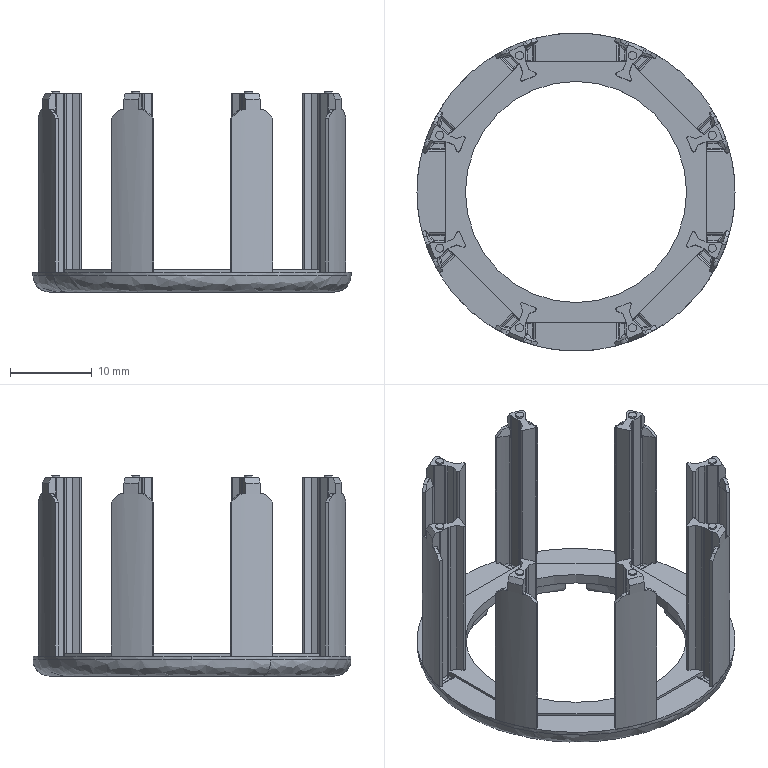Part | STEP file | TQ-DD-1105-THMagnetHolder1010_デフォルト | 1 solid | 542 faces | box 38.83 x 38.83 x 24.45 mm | volume 2757 mm3 | cylinder 232 | plane 220 | spline 66 | cone 24 | commonest cylinder face diameters 0.4 x86 1 x40 0.6 x36 0.2 x18 2 x16 21 x16